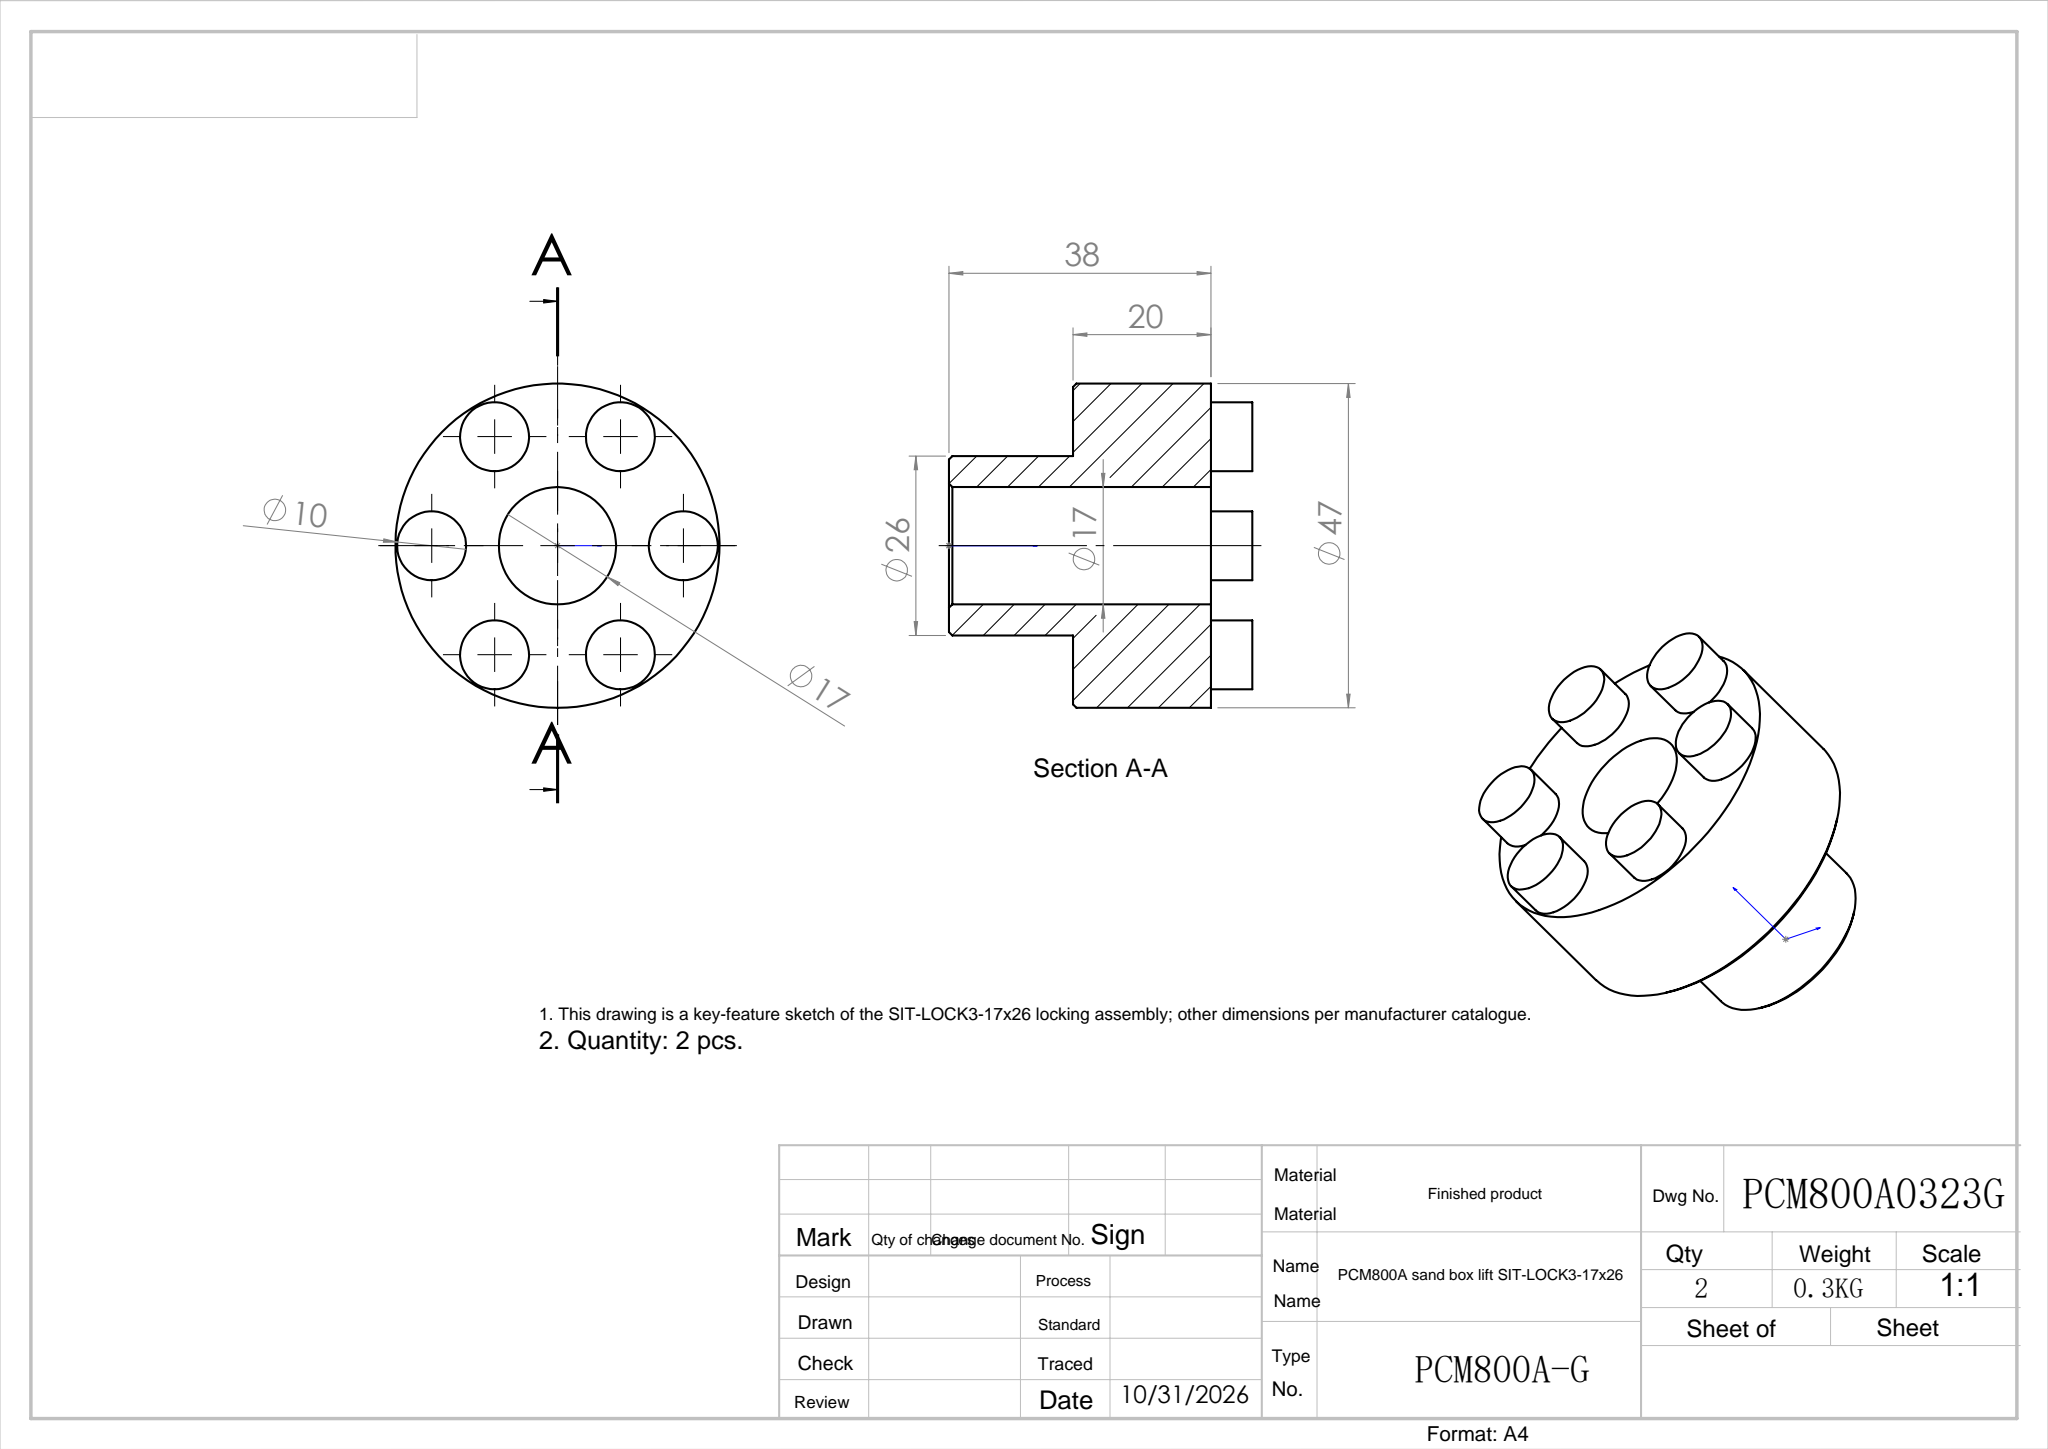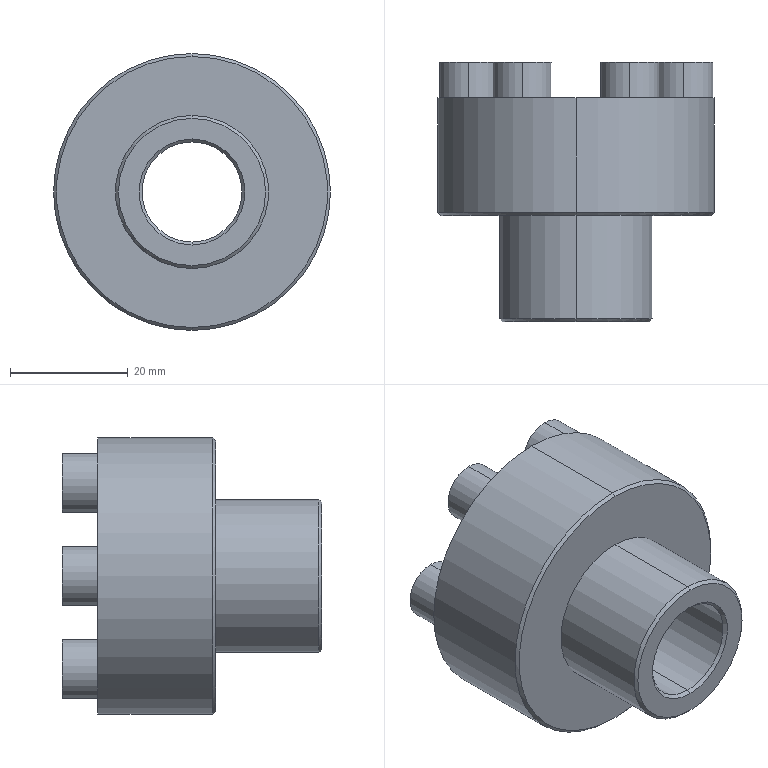Part | SolidWorks | features Boss 2, Chamfer 1, Cut 1, Extrusion 1 | 1 solid | 33 faces | box 47 x 44 x 47 mm | volume 38423 mm3 | cylinder 18 | plane 9 | cone 6 | commonest cylinder face diameters 10 x12 17 x2 26 x2 47 x2
STEP:
#1=CARTESIAN_POINT('',(0.,0.5,8.5));
#2=VERTEX_POINT('',#1);
#3=CARTESIAN_POINT('',(0.,0.5,-8.5));
#4=VERTEX_POINT('',#3);
#5=CARTESIAN_POINT('',(0.,0.5,0.));
#6=DIRECTION('',(0.,-1.,0.));
#7=DIRECTION('',(0.,0.,1.));
#8=AXIS2_PLACEMENT_3D('',#5,#6,#7);
#9=CIRCLE('',#8,8.5);
#10=EDGE_CURVE('',#2,#4,#9,.T.);
#11=ORIENTED_EDGE('',*,*,#10,.F.);
#12=CARTESIAN_POINT('',(0.,0.,9.));
#13=VERTEX_POINT('',#12);
#14=CARTESIAN_POINT('',(0.,0.,9.));
#15=DIRECTION('',(0.,-0.7071,0.7071));
#16=VECTOR('',#15,1000.);
#17=LINE('',#14,#16);
#18=EDGE_CURVE('',#2,#13,#17,.T.);
#19=ORIENTED_EDGE('',*,*,#18,.T.);
#20=CARTESIAN_POINT('',(0.,0.,-9.));
#21=VERTEX_POINT('',#20);
#22=CARTESIAN_POINT('',(0.,0.,0.));
#23=DIRECTION('',(0.,1.,0.));
#24=DIRECTION('',(0.,0.,1.));
#25=AXIS2_PLACEMENT_3D('',#22,#23,#24);
#26=CIRCLE('',#25,9.);
#27=EDGE_CURVE('',#21,#13,#26,.T.);
#28=ORIENTED_EDGE('',*,*,#27,.F.);
#29=CARTESIAN_POINT('',(0.,0.,-9.));
#30=DIRECTION('',(0.,-0.7071,-0.7071));
#31=VECTOR('',#30,1000.);
#32=LINE('',#29,#31);
#33=EDGE_CURVE('',#4,#21,#32,.T.);
#34=ORIENTED_EDGE('',*,*,#33,.F.);
#35=EDGE_LOOP('',(#11,#19,#28,#34));
#36=FACE_OUTER_BOUND('',#35,.T.);
#37=CARTESIAN_POINT('',(0.,0.,0.));
#38=DIRECTION('',(0.,-1.,0.));
#39=DIRECTION('',(0.,0.,-1.));
#40=AXIS2_PLACEMENT_3D('',#37,#38,#39);
#41=CONICAL_SURFACE('',#40,9.,0.7854);
#42=ADVANCED_FACE('',(#36),#41,.F.);
#43=CARTESIAN_POINT('',(0.,0.,-12.5));
#44=VERTEX_POINT('',#43);
#45=CARTESIAN_POINT('',(0.,0.,12.5));
#46=VERTEX_POINT('',#45);
#47=CARTESIAN_POINT('',(0.,0.,0.));
#48=DIRECTION('',(0.,-1.,0.));
#49=DIRECTION('',(0.,0.,1.));
#50=AXIS2_PLACEMENT_3D('',#47,#48,#49);
#51=CIRCLE('',#50,12.5);
#52=EDGE_CURVE('',#44,#46,#51,.T.);
#53=ORIENTED_EDGE('',*,*,#52,.F.);
#54=CARTESIAN_POINT('',(0.,0.5,-13.));
#55=VERTEX_POINT('',#54);
#56=CARTESIAN_POINT('',(0.,0.5,-13.));
#57=DIRECTION('',(0.,0.7071,-0.7071));
#58=VECTOR('',#57,1000.);
#59=LINE('',#56,#58);
#60=EDGE_CURVE('',#44,#55,#59,.T.);
#61=ORIENTED_EDGE('',*,*,#60,.T.);
#62=CARTESIAN_POINT('',(0.,0.5,13.));
#63=VERTEX_POINT('',#62);
#64=CARTESIAN_POINT('',(0.,0.5,0.));
#65=DIRECTION('',(0.,1.,0.));
#66=DIRECTION('',(0.,0.,1.));
#67=AXIS2_PLACEMENT_3D('',#64,#65,#66);
#68=CIRCLE('',#67,13.);
#69=EDGE_CURVE('',#63,#55,#68,.T.);
#70=ORIENTED_EDGE('',*,*,#69,.F.);
#71=CARTESIAN_POINT('',(0.,0.5,13.));
#72=DIRECTION('',(0.,0.7071,0.7071));
#73=VECTOR('',#72,1000.);
#74=LINE('',#71,#73);
#75=EDGE_CURVE('',#46,#63,#74,.T.);
#76=ORIENTED_EDGE('',*,*,#75,.F.);
#77=EDGE_LOOP('',(#53,#61,#70,#76));
#78=FACE_OUTER_BOUND('',#77,.T.);
#79=CARTESIAN_POINT('',(0.,0.5,0.));
#80=DIRECTION('',(0.,1.,0.));
#81=DIRECTION('',(0.,0.,1.));
#82=AXIS2_PLACEMENT_3D('',#79,#80,#81);
#83=CONICAL_SURFACE('',#82,13.,0.7854);
#84=ADVANCED_FACE('',(#78),#83,.T.);
#85=CARTESIAN_POINT('',(0.,18.,-23.));
#86=VERTEX_POINT('',#85);
#87=CARTESIAN_POINT('',(0.,18.,23.));
#88=VERTEX_POINT('',#87);
#89=CARTESIAN_POINT('',(0.,18.,0.));
#90=DIRECTION('',(0.,-1.,0.));
#91=DIRECTION('',(0.,0.,1.));
#92=AXIS2_PLACEMENT_3D('',#89,#90,#91);
#93=CIRCLE('',#92,23.);
#94=EDGE_CURVE('',#86,#88,#93,.T.);
#95=ORIENTED_EDGE('',*,*,#94,.F.);
#96=CARTESIAN_POINT('',(0.,18.5,-23.5));
#97=VERTEX_POINT('',#96);
#98=CARTESIAN_POINT('',(0.,18.5,-23.5));
#99=DIRECTION('',(0.,0.7071,-0.7071));
#100=VECTOR('',#99,1000.);
#101=LINE('',#98,#100);
#102=EDGE_CURVE('',#86,#97,#101,.T.);
#103=ORIENTED_EDGE('',*,*,#102,.T.);
#104=CARTESIAN_POINT('',(0.,18.5,23.5));
#105=VERTEX_POINT('',#104);
#106=CARTESIAN_POINT('',(0.,18.5,0.));
#107=DIRECTION('',(0.,1.,0.));
#108=DIRECTION('',(0.,0.,1.));
#109=AXIS2_PLACEMENT_3D('',#106,#107,#108);
#110=CIRCLE('',#109,23.5);
#111=EDGE_CURVE('',#105,#97,#110,.T.);
#112=ORIENTED_EDGE('',*,*,#111,.F.);
#113=CARTESIAN_POINT('',(0.,18.5,23.5));
#114=DIRECTION('',(0.,0.7071,0.7071));
#115=VECTOR('',#114,1000.);
#116=LINE('',#113,#115);
#117=EDGE_CURVE('',#88,#105,#116,.T.);
#118=ORIENTED_EDGE('',*,*,#117,.F.);
#119=EDGE_LOOP('',(#95,#103,#112,#118));
#120=FACE_OUTER_BOUND('',#119,.T.);
#121=CARTESIAN_POINT('',(0.,18.5,0.));
#122=DIRECTION('',(0.,1.,0.));
#123=DIRECTION('',(0.,0.,1.));
#124=AXIS2_PLACEMENT_3D('',#121,#122,#123);
#125=CONICAL_SURFACE('',#124,23.5,0.7854);
#126=ADVANCED_FACE('',(#120),#125,.T.);
#127=CARTESIAN_POINT('',(9.125,44.,-10.805));
#128=VERTEX_POINT('',#127);
#129=CARTESIAN_POINT('',(9.125,44.,-20.805));
#130=VERTEX_POINT('',#129);
#131=CARTESIAN_POINT('',(9.125,44.,-15.805));
#132=DIRECTION('',(0.,1.,0.));
#133=DIRECTION('',(0.,0.,1.));
#134=AXIS2_PLACEMENT_3D('',#131,#132,#133);
#135=CIRCLE('',#134,5.);
#136=EDGE_CURVE('',#128,#130,#135,.T.);
#137=ORIENTED_EDGE('',*,*,#136,.F.);
#138=CARTESIAN_POINT('',(9.125,38.,-10.805));
#139=VERTEX_POINT('',#138);
#140=CARTESIAN_POINT('',(9.125,44.,-10.805));
#141=DIRECTION('',(0.,-1.,0.));
#142=VECTOR('',#141,1000.);
#143=LINE('',#140,#142);
#144=EDGE_CURVE('',#128,#139,#143,.T.);
#145=ORIENTED_EDGE('',*,*,#144,.T.);
#146=CARTESIAN_POINT('',(9.125,38.,-20.805));
#147=VERTEX_POINT('',#146);
#148=CARTESIAN_POINT('',(9.125,38.,-15.805));
#149=DIRECTION('',(0.,1.,0.));
#150=DIRECTION('',(0.,0.,1.));
#151=AXIS2_PLACEMENT_3D('',#148,#149,#150);
#152=CIRCLE('',#151,5.);
#153=EDGE_CURVE('',#139,#147,#152,.T.);
#154=ORIENTED_EDGE('',*,*,#153,.T.);
#155=CARTESIAN_POINT('',(9.125,44.,-20.805));
#156=DIRECTION('',(0.,-1.,0.));
#157=VECTOR('',#156,1000.);
#158=LINE('',#155,#157);
#159=EDGE_CURVE('',#130,#147,#158,.T.);
#160=ORIENTED_EDGE('',*,*,#159,.F.);
#161=EDGE_LOOP('',(#137,#145,#154,#160));
#162=FACE_OUTER_BOUND('',#161,.T.);
#163=CARTESIAN_POINT('',(9.125,44.,-15.805));
#164=DIRECTION('',(0.,-1.,0.));
#165=DIRECTION('',(0.,0.,-1.));
#166=AXIS2_PLACEMENT_3D('',#163,#164,#165);
#167=CYLINDRICAL_SURFACE('',#166,5.);
#168=ADVANCED_FACE('',(#162),#167,.T.);
#169=CARTESIAN_POINT('',(-9.125,44.,-10.805));
#170=VERTEX_POINT('',#169);
#171=CARTESIAN_POINT('',(-9.125,44.,-20.805));
#172=VERTEX_POINT('',#171);
#173=CARTESIAN_POINT('',(-9.125,44.,-15.805));
#174=DIRECTION('',(0.,1.,0.));
#175=DIRECTION('',(0.,0.,1.));
#176=AXIS2_PLACEMENT_3D('',#173,#174,#175);
#177=CIRCLE('',#176,5.);
#178=EDGE_CURVE('',#170,#172,#177,.T.);
#179=ORIENTED_EDGE('',*,*,#178,.F.);
#180=CARTESIAN_POINT('',(-9.125,38.,-10.805));
#181=VERTEX_POINT('',#180);
#182=CARTESIAN_POINT('',(-9.125,44.,-10.805));
#183=DIRECTION('',(0.,-1.,0.));
#184=VECTOR('',#183,1000.);
#185=LINE('',#182,#184);
#186=EDGE_CURVE('',#170,#181,#185,.T.);
#187=ORIENTED_EDGE('',*,*,#186,.T.);
#188=CARTESIAN_POINT('',(-9.125,38.,-20.805));
#189=VERTEX_POINT('',#188);
#190=CARTESIAN_POINT('',(-9.125,38.,-15.805));
#191=DIRECTION('',(0.,1.,0.));
#192=DIRECTION('',(0.,0.,1.));
#193=AXIS2_PLACEMENT_3D('',#190,#191,#192);
#194=CIRCLE('',#193,5.);
#195=EDGE_CURVE('',#181,#189,#194,.T.);
#196=ORIENTED_EDGE('',*,*,#195,.T.);
#197=CARTESIAN_POINT('',(-9.125,44.,-20.805));
#198=DIRECTION('',(0.,-1.,0.));
#199=VECTOR('',#198,1000.);
#200=LINE('',#197,#199);
#201=EDGE_CURVE('',#172,#189,#200,.T.);
#202=ORIENTED_EDGE('',*,*,#201,.F.);
#203=EDGE_LOOP('',(#179,#187,#196,#202));
#204=FACE_OUTER_BOUND('',#203,.T.);
#205=CARTESIAN_POINT('',(-9.125,44.,-15.805));
#206=DIRECTION('',(0.,-1.,0.));
#207=DIRECTION('',(0.,0.,-1.));
#208=AXIS2_PLACEMENT_3D('',#205,#206,#207);
#209=CYLINDRICAL_SURFACE('',#208,5.);
#210=ADVANCED_FACE('',(#204),#209,.T.);
#211=CARTESIAN_POINT('',(-18.25,44.,5.));
#212=VERTEX_POINT('',#211);
#213=CARTESIAN_POINT('',(-18.25,44.,-5.));
#214=VERTEX_POINT('',#213);
#215=CARTESIAN_POINT('',(-18.25,44.,0.));
#216=DIRECTION('',(0.,1.,0.));
#217=DIRECTION('',(0.,0.,1.));
#218=AXIS2_PLACEMENT_3D('',#215,#216,#217);
#219=CIRCLE('',#218,5.);
#220=EDGE_CURVE('',#212,#214,#219,.T.);
#221=ORIENTED_EDGE('',*,*,#220,.F.);
#222=CARTESIAN_POINT('',(-18.25,38.,5.));
#223=VERTEX_POINT('',#222);
#224=CARTESIAN_POINT('',(-18.25,44.,5.));
#225=DIRECTION('',(0.,-1.,0.));
#226=VECTOR('',#225,1000.);
#227=LINE('',#224,#226);
#228=EDGE_CURVE('',#212,#223,#227,.T.);
#229=ORIENTED_EDGE('',*,*,#228,.T.);
#230=CARTESIAN_POINT('',(-18.25,38.,-5.));
#231=VERTEX_POINT('',#230);
#232=CARTESIAN_POINT('',(-18.25,38.,0.));
#233=DIRECTION('',(0.,1.,0.));
#234=DIRECTION('',(0.,0.,1.));
#235=AXIS2_PLACEMENT_3D('',#232,#233,#234);
#236=CIRCLE('',#235,5.);
#237=EDGE_CURVE('',#223,#231,#236,.T.);
#238=ORIENTED_EDGE('',*,*,#237,.T.);
#239=CARTESIAN_POINT('',(-18.25,44.,-5.));
#240=DIRECTION('',(0.,-1.,0.));
#241=VECTOR('',#240,1000.);
#242=LINE('',#239,#241);
#243=EDGE_CURVE('',#214,#231,#242,.T.);
#244=ORIENTED_EDGE('',*,*,#243,.F.);
#245=EDGE_LOOP('',(#221,#229,#238,#244));
#246=FACE_OUTER_BOUND('',#245,.T.);
#247=CARTESIAN_POINT('',(-18.25,44.,0.));
#248=DIRECTION('',(0.,-1.,0.));
#249=DIRECTION('',(0.,0.,-1.));
#250=AXIS2_PLACEMENT_3D('',#247,#248,#249);
#251=CYLINDRICAL_SURFACE('',#250,5.);
#252=ADVANCED_FACE('',(#246),#251,.T.);
#253=CARTESIAN_POINT('',(-9.125,44.,20.805));
#254=VERTEX_POINT('',#253);
#255=CARTESIAN_POINT('',(-9.125,44.,10.805));
#256=VERTEX_POINT('',#255);
#257=CARTESIAN_POINT('',(-9.125,44.,15.805));
#258=DIRECTION('',(0.,1.,0.));
#259=DIRECTION('',(0.,0.,1.));
#260=AXIS2_PLACEMENT_3D('',#257,#258,#259);
#261=CIRCLE('',#260,5.);
#262=EDGE_CURVE('',#254,#256,#261,.T.);
#263=ORIENTED_EDGE('',*,*,#262,.F.);
#264=CARTESIAN_POINT('',(-9.125,38.,20.805));
#265=VERTEX_POINT('',#264);
#266=CARTESIAN_POINT('',(-9.125,44.,20.805));
#267=DIRECTION('',(0.,-1.,0.));
#268=VECTOR('',#267,1000.);
#269=LINE('',#266,#268);
#270=EDGE_CURVE('',#254,#265,#269,.T.);
#271=ORIENTED_EDGE('',*,*,#270,.T.);
#272=CARTESIAN_POINT('',(-9.125,38.,10.805));
#273=VERTEX_POINT('',#272);
#274=CARTESIAN_POINT('',(-9.125,38.,15.805));
#275=DIRECTION('',(0.,1.,0.));
#276=DIRECTION('',(0.,0.,1.));
#277=AXIS2_PLACEMENT_3D('',#274,#275,#276);
#278=CIRCLE('',#277,5.);
#279=EDGE_CURVE('',#265,#273,#278,.T.);
#280=ORIENTED_EDGE('',*,*,#279,.T.);
#281=CARTESIAN_POINT('',(-9.125,44.,10.805));
#282=DIRECTION('',(0.,-1.,0.));
#283=VECTOR('',#282,1000.);
#284=LINE('',#281,#283);
#285=EDGE_CURVE('',#256,#273,#284,.T.);
#286=ORIENTED_EDGE('',*,*,#285,.F.);
#287=EDGE_LOOP('',(#263,#271,#280,#286));
#288=FACE_OUTER_BOUND('',#287,.T.);
#289=CARTESIAN_POINT('',(-9.125,44.,15.805));
#290=DIRECTION('',(0.,-1.,0.));
#291=DIRECTION('',(0.,0.,-1.));
#292=AXIS2_PLACEMENT_3D('',#289,#290,#291);
#293=CYLINDRICAL_SURFACE('',#292,5.);
#294=ADVANCED_FACE('',(#288),#293,.T.);
#295=CARTESIAN_POINT('',(9.125,44.,20.805));
#296=VERTEX_POINT('',#295);
#297=CARTESIAN_POINT('',(9.125,44.,10.805));
#298=VERTEX_POINT('',#297);
#299=CARTESIAN_POINT('',(9.125,44.,15.805));
#300=DIRECTION('',(0.,1.,0.));
#301=DIRECTION('',(0.,0.,1.));
#302=AXIS2_PLACEMENT_3D('',#299,#300,#301);
#303=CIRCLE('',#302,5.);
#304=EDGE_CURVE('',#296,#298,#303,.T.);
#305=ORIENTED_EDGE('',*,*,#304,.F.);
#306=CARTESIAN_POINT('',(9.125,38.,20.805));
#307=VERTEX_POINT('',#306);
#308=CARTESIAN_POINT('',(9.125,44.,20.805));
#309=DIRECTION('',(0.,-1.,0.));
#310=VECTOR('',#309,1000.);
#311=LINE('',#308,#310);
#312=EDGE_CURVE('',#296,#307,#311,.T.);
#313=ORIENTED_EDGE('',*,*,#312,.T.);
#314=CARTESIAN_POINT('',(9.125,38.,10.805));
#315=VERTEX_POINT('',#314);
#316=CARTESIAN_POINT('',(9.125,38.,15.805));
#317=DIRECTION('',(0.,1.,0.));
#318=DIRECTION('',(0.,0.,1.));
#319=AXIS2_PLACEMENT_3D('',#316,#317,#318);
#320=CIRCLE('',#319,5.);
#321=EDGE_CURVE('',#307,#315,#320,.T.);
#322=ORIENTED_EDGE('',*,*,#321,.T.);
#323=CARTESIAN_POINT('',(9.125,44.,10.805));
#324=DIRECTION('',(0.,-1.,0.));
#325=VECTOR('',#324,1000.);
#326=LINE('',#323,#325);
#327=EDGE_CURVE('',#298,#315,#326,.T.);
#328=ORIENTED_EDGE('',*,*,#327,.F.);
#329=EDGE_LOOP('',(#305,#313,#322,#328));
#330=FACE_OUTER_BOUND('',#329,.T.);
#331=CARTESIAN_POINT('',(9.125,44.,15.805));
#332=DIRECTION('',(0.,-1.,0.));
#333=DIRECTION('',(0.,0.,-1.));
#334=AXIS2_PLACEMENT_3D('',#331,#332,#333);
#335=CYLINDRICAL_SURFACE('',#334,5.);
#336=ADVANCED_FACE('',(#330),#335,.T.);
#337=CARTESIAN_POINT('',(18.25,44.,5.));
#338=VERTEX_POINT('',#337);
#339=CARTESIAN_POINT('',(18.25,44.,-5.));
#340=VERTEX_POINT('',#339);
#341=CARTESIAN_POINT('',(18.25,44.,0.));
#342=DIRECTION('',(0.,1.,0.));
#343=DIRECTION('',(0.,0.,1.));
#344=AXIS2_PLACEMENT_3D('',#341,#342,#343);
#345=CIRCLE('',#344,5.);
#346=EDGE_CURVE('',#338,#340,#345,.T.);
#347=ORIENTED_EDGE('',*,*,#346,.F.);
#348=CARTESIAN_POINT('',(18.25,38.,5.));
#349=VERTEX_POINT('',#348);
#350=CARTESIAN_POINT('',(18.25,44.,5.));
#351=DIRECTION('',(0.,-1.,0.));
#352=VECTOR('',#351,1000.);
#353=LINE('',#350,#352);
#354=EDGE_CURVE('',#338,#349,#353,.T.);
#355=ORIENTED_EDGE('',*,*,#354,.T.);
#356=CARTESIAN_POINT('',(18.25,38.,-5.));
#357=VERTEX_POINT('',#356);
#358=CARTESIAN_POINT('',(18.25,38.,0.));
#359=DIRECTION('',(0.,1.,0.));
#360=DIRECTION('',(0.,0.,1.));
#361=AXIS2_PLACEMENT_3D('',#358,#359,#360);
#362=CIRCLE('',#361,5.);
#363=EDGE_CURVE('',#349,#357,#362,.T.);
#364=ORIENTED_EDGE('',*,*,#363,.T.);
#365=CARTESIAN_POINT('',(18.25,44.,-5.));
#366=DIRECTION('',(0.,-1.,0.));
#367=VECTOR('',#366,1000.);
#368=LINE('',#365,#367);
#369=EDGE_CURVE('',#340,#357,#368,.T.);
#370=ORIENTED_EDGE('',*,*,#369,.F.);
#371=EDGE_LOOP('',(#347,#355,#364,#370));
#372=FACE_OUTER_BOUND('',#371,.T.);
#373=CARTESIAN_POINT('',(18.25,44.,0.));
#374=DIRECTION('',(0.,-1.,0.));
#375=DIRECTION('',(0.,0.,-1.));
#376=AXIS2_PLACEMENT_3D('',#373,#374,#375);
#377=CYLINDRICAL_SURFACE('',#376,5.);
#378=ADVANCED_FACE('',(#372),#377,.T.);
#379=CARTESIAN_POINT('',(0.,38.,23.5));
#380=VERTEX_POINT('',#379);
#381=CARTESIAN_POINT('',(0.,38.,-23.5));
#382=VERTEX_POINT('',#381);
#383=CARTESIAN_POINT('',(0.,38.,0.));
#384=DIRECTION('',(0.,1.,0.));
#385=DIRECTION('',(0.,0.,1.));
#386=AXIS2_PLACEMENT_3D('',#383,#384,#385);
#387=CIRCLE('',#386,23.5);
#388=EDGE_CURVE('',#380,#382,#387,.T.);
#389=ORIENTED_EDGE('',*,*,#388,.F.);
#390=CARTESIAN_POINT('',(0.,38.,23.5));
#391=DIRECTION('',(0.,-1.,0.));
#392=VECTOR('',#391,1000.);
#393=LINE('',#390,#392);
#394=EDGE_CURVE('',#380,#105,#393,.T.);
#395=ORIENTED_EDGE('',*,*,#394,.T.);
#396=ORIENTED_EDGE('',*,*,#111,.T.);
#397=CARTESIAN_POINT('',(0.,38.,-23.5));
#398=DIRECTION('',(0.,-1.,0.));
#399=VECTOR('',#398,1000.);
#400=LINE('',#397,#399);
#401=EDGE_CURVE('',#382,#97,#400,.T.);
#402=ORIENTED_EDGE('',*,*,#401,.F.);
#403=EDGE_LOOP('',(#389,#395,#396,#402));
#404=FACE_OUTER_BOUND('',#403,.T.);
#405=CARTESIAN_POINT('',(0.,38.,0.));
#406=DIRECTION('',(0.,-1.,0.));
#407=DIRECTION('',(0.,0.,-1.));
#408=AXIS2_PLACEMENT_3D('',#405,#406,#407);
#409=CYLINDRICAL_SURFACE('',#408,23.5);
#410=ADVANCED_FACE('',(#404),#409,.T.);
#411=CARTESIAN_POINT('',(0.,38.,8.5));
#412=VERTEX_POINT('',#411);
#413=CARTESIAN_POINT('',(0.,38.,-8.5));
#414=VERTEX_POINT('',#413);
#415=CARTESIAN_POINT('',(0.,38.,0.));
#416=DIRECTION('',(0.,-1.,0.));
#417=DIRECTION('',(0.,0.,-1.));
#418=AXIS2_PLACEMENT_3D('',#415,#416,#417);
#419=CIRCLE('',#418,8.5);
#420=EDGE_CURVE('',#412,#414,#419,.T.);
#421=ORIENTED_EDGE('',*,*,#420,.F.);
#422=CARTESIAN_POINT('',(0.,18.,8.5));
#423=DIRECTION('',(0.,-1.,0.));
#424=VECTOR('',#423,1000.);
#425=LINE('',#422,#424);
#426=EDGE_CURVE('',#412,#2,#425,.T.);
#427=ORIENTED_EDGE('',*,*,#426,.T.);
#428=ORIENTED_EDGE('',*,*,#10,.T.);
#429=CARTESIAN_POINT('',(0.,18.,-8.5));
#430=DIRECTION('',(0.,-1.,0.));
#431=VECTOR('',#430,1000.);
#432=LINE('',#429,#431);
#433=EDGE_CURVE('',#414,#4,#432,.T.);
#434=ORIENTED_EDGE('',*,*,#433,.F.);
#435=EDGE_LOOP('',(#421,#427,#428,#434));
#436=FACE_OUTER_BOUND('',#435,.T.);
#437=CARTESIAN_POINT('',(0.,18.,0.));
#438=DIRECTION('',(0.,-1.,0.));
#439=DIRECTION('',(0.,0.,-1.));
#440=AXIS2_PLACEMENT_3D('',#437,#438,#439);
#441=CYLINDRICAL_SURFACE('',#440,8.5);
#442=ADVANCED_FACE('',(#436),#441,.F.);
#443=CARTESIAN_POINT('',(0.,18.,13.));
#444=VERTEX_POINT('',#443);
#445=CARTESIAN_POINT('',(0.,18.,-13.));
#446=VERTEX_POINT('',#445);
#447=CARTESIAN_POINT('',(0.,18.,0.));
#448=DIRECTION('',(0.,1.,0.));
#449=DIRECTION('',(0.,0.,1.));
#450=AXIS2_PLACEMENT_3D('',#447,#448,#449);
#451=CIRCLE('',#450,13.);
#452=EDGE_CURVE('',#444,#446,#451,.T.);
#453=ORIENTED_EDGE('',*,*,#452,.F.);
#454=CARTESIAN_POINT('',(0.,18.,13.));
#455=DIRECTION('',(0.,-1.,0.));
#456=VECTOR('',#455,1000.);
#457=LINE('',#454,#456);
#458=EDGE_CURVE('',#444,#63,#457,.T.);
#459=ORIENTED_EDGE('',*,*,#458,.T.);
#460=ORIENTED_EDGE('',*,*,#69,.T.);
#461=CARTESIAN_POINT('',(0.,18.,-13.));
#462=DIRECTION('',(0.,-1.,0.));
#463=VECTOR('',#462,1000.);
#464=LINE('',#461,#463);
#465=EDGE_CURVE('',#446,#55,#464,.T.);
#466=ORIENTED_EDGE('',*,*,#465,.F.);
#467=EDGE_LOOP('',(#453,#459,#460,#466));
#468=FACE_OUTER_BOUND('',#467,.T.);
#469=CARTESIAN_POINT('',(0.,18.,0.));
#470=DIRECTION('',(0.,-1.,0.));
#471=DIRECTION('',(0.,0.,-1.));
#472=AXIS2_PLACEMENT_3D('',#469,#470,#471);
#473=CYLINDRICAL_SURFACE('',#472,13.);
#474=ADVANCED_FACE('',(#468),#473,.T.);
#475=CARTESIAN_POINT('',(-9.125,38.,-15.805));
#476=DIRECTION('',(0.,1.,0.));
#477=DIRECTION('',(0.,0.,1.));
#478=AXIS2_PLACEMENT_3D('',#475,#476,#477);
#479=CIRCLE('',#478,5.);
#480=EDGE_CURVE('',#189,#181,#479,.T.);
#481=ORIENTED_EDGE('',*,*,#480,.F.);
#482=ORIENTED_EDGE('',*,*,#195,.F.);
#483=EDGE_LOOP('',(#481,#482));
#484=FACE_BOUND('',#483,.T.);
#485=CARTESIAN_POINT('',(-9.125,38.,15.805));
#486=DIRECTION('',(0.,1.,0.));
#487=DIRECTION('',(0.,0.,1.));
#488=AXIS2_PLACEMENT_3D('',#485,#486,#487);
#489=CIRCLE('',#488,5.);
#490=EDGE_CURVE('',#273,#265,#489,.T.);
#491=ORIENTED_EDGE('',*,*,#490,.F.);
#492=ORIENTED_EDGE('',*,*,#279,.F.);
#493=EDGE_LOOP('',(#491,#492));
#494=FACE_BOUND('',#493,.T.);
#495=CARTESIAN_POINT('',(18.25,38.,0.));
#496=DIRECTION('',(0.,1.,0.));
#497=DIRECTION('',(0.,0.,1.));
#498=AXIS2_PLACEMENT_3D('',#495,#496,#497);
#499=CIRCLE('',#498,5.);
#500=EDGE_CURVE('',#357,#349,#499,.T.);
#501=ORIENTED_EDGE('',*,*,#500,.F.);
#502=ORIENTED_EDGE('',*,*,#363,.F.);
#503=EDGE_LOOP('',(#501,#502));
#504=FACE_BOUND('',#503,.T.);
#505=CARTESIAN_POINT('',(0.,38.,0.));
#506=DIRECTION('',(0.,-1.,0.));
#507=DIRECTION('',(0.,0.,-1.));
#508=AXIS2_PLACEMENT_3D('',#505,#506,#507);
#509=CIRCLE('',#508,8.5);
#510=EDGE_CURVE('',#414,#412,#509,.T.);
#511=ORIENTED_EDGE('',*,*,#510,.T.);
#512=ORIENTED_EDGE('',*,*,#420,.T.);
#513=EDGE_LOOP('',(#511,#512));
#514=FACE_BOUND('',#513,.T.);
#515=CARTESIAN_POINT('',(0.,38.,0.));
#516=DIRECTION('',(0.,1.,0.));
#517=DIRECTION('',(0.,0.,1.));
#518=AXIS2_PLACEMENT_3D('',#515,#516,#517);
#519=CIRCLE('',#518,23.5);
#520=EDGE_CURVE('',#382,#380,#519,.T.);
#521=ORIENTED_EDGE('',*,*,#520,.T.);
#522=ORIENTED_EDGE('',*,*,#388,.T.);
#523=EDGE_LOOP('',(#521,#522));
#524=FACE_OUTER_BOUND('',#523,.T.);
#525=CARTESIAN_POINT('',(9.125,38.,15.805));
#526=DIRECTION('',(0.,1.,0.));
#527=DIRECTION('',(0.,0.,1.));
#528=AXIS2_PLACEMENT_3D('',#525,#526,#527);
#529=CIRCLE('',#528,5.);
#530=EDGE_CURVE('',#315,#307,#529,.T.);
#531=ORIENTED_EDGE('',*,*,#530,.F.);
#532=ORIENTED_EDGE('',*,*,#321,.F.);
#533=EDGE_LOOP('',(#531,#532));
#534=FACE_BOUND('',#533,.T.);
#535=CARTESIAN_POINT('',(-18.25,38.,0.));
#536=DIRECTION('',(0.,1.,0.));
#537=DIRECTION('',(0.,0.,1.));
#538=AXIS2_PLACEMENT_3D('',#535,#536,#537);
#539=CIRCLE('',#538,5.);
#540=EDGE_CURVE('',#231,#223,#539,.T.);
#541=ORIENTED_EDGE('',*,*,#540,.F.);
#542=ORIENTED_EDGE('',*,*,#237,.F.);
#543=EDGE_LOOP('',(#541,#542));
#544=FACE_BOUND('',#543,.T.);
#545=CARTESIAN_POINT('',(9.125,38.,-15.805));
#546=DIRECTION('',(0.,1.,0.));
#547=DIRECTION('',(0.,0.,1.));
#548=AXIS2_PLACEMENT_3D('',#545,#546,#547);
#549=CIRCLE('',#548,5.);
#550=EDGE_CURVE('',#147,#139,#549,.T.);
#551=ORIENTED_EDGE('',*,*,#550,.F.);
#552=ORIENTED_EDGE('',*,*,#153,.F.);
#553=EDGE_LOOP('',(#551,#552));
#554=FACE_BOUND('',#553,.T.);
#555=CARTESIAN_POINT('',(0.,38.,0.));
#556=DIRECTION('',(0.,1.,0.));
#557=DIRECTION('',(0.,0.,1.));
#558=AXIS2_PLACEMENT_3D('',#555,#556,#557);
#559=PLANE('',#558);
#560=ADVANCED_FACE('',(#484,#494,#504,#514,#524,#534,#544,#554),#559,.T.);
#561=CARTESIAN_POINT('',(0.,0.,0.));
#562=DIRECTION('',(0.,-1.,0.));
#563=DIRECTION('',(0.,0.,1.));
#564=AXIS2_PLACEMENT_3D('',#561,#562,#563);
#565=CIRCLE('',#564,12.5);
#566=EDGE_CURVE('',#46,#44,#565,.T.);
#567=ORIENTED_EDGE('',*,*,#566,.T.);
#568=ORIENTED_EDGE('',*,*,#52,.T.);
#569=EDGE_LOOP('',(#567,#568));
#570=FACE_OUTER_BOUND('',#569,.T.);
#571=ORIENTED_EDGE('',*,*,#27,.T.);
#572=CARTESIAN_POINT('',(0.,0.,0.));
#573=DIRECTION('',(0.,1.,0.));
#574=DIRECTION('',(0.,0.,1.));
#575=AXIS2_PLACEMENT_3D('',#572,#573,#574);
#576=CIRCLE('',#575,9.);
#577=EDGE_CURVE('',#13,#21,#576,.T.);
#578=ORIENTED_EDGE('',*,*,#577,.T.);
#579=EDGE_LOOP('',(#571,#578));
#580=FACE_BOUND('',#579,.T.);
#581=CARTESIAN_POINT('',(0.,0.,0.));
#582=DIRECTION('',(0.,1.,0.));
#583=DIRECTION('',(0.,0.,1.));
#584=AXIS2_PLACEMENT_3D('',#581,#582,#583);
#585=PLANE('',#584);
#586=ADVANCED_FACE('',(#570,#580),#585,.F.);
#587=ORIENTED_EDGE('',*,*,#458,.F.);
#588=CARTESIAN_POINT('',(0.,18.,0.));
#589=DIRECTION('',(0.,1.,0.));
#590=DIRECTION('',(0.,0.,1.));
#591=AXIS2_PLACEMENT_3D('',#588,#589,#590);
#592=CIRCLE('',#591,13.);
#593=EDGE_CURVE('',#446,#444,#592,.T.);
#594=ORIENTED_EDGE('',*,*,#593,.F.);
#595=ORIENTED_EDGE('',*,*,#465,.T.);
#596=CARTESIAN_POINT('',(0.,0.5,0.));
#597=DIRECTION('',(0.,1.,0.));
#598=DIRECTION('',(0.,0.,1.));
#599=AXIS2_PLACEMENT_3D('',#596,#597,#598);
#600=CIRCLE('',#599,13.);
#601=EDGE_CURVE('',#55,#63,#600,.T.);
#602=ORIENTED_EDGE('',*,*,#601,.T.);
#603=EDGE_LOOP('',(#587,#594,#595,#602));
#604=FACE_OUTER_BOUND('',#603,.T.);
#605=CARTESIAN_POINT('',(0.,18.,0.));
#606=DIRECTION('',(0.,-1.,0.));
#607=DIRECTION('',(0.,0.,-1.));
#608=AXIS2_PLACEMENT_3D('',#605,#606,#607);
#609=CYLINDRICAL_SURFACE('',#608,13.);
#610=ADVANCED_FACE('',(#604),#609,.T.);
#611=ORIENTED_EDGE('',*,*,#426,.F.);
#612=ORIENTED_EDGE('',*,*,#510,.F.);
#613=ORIENTED_EDGE('',*,*,#433,.T.);
#614=CARTESIAN_POINT('',(0.,0.5,0.));
#615=DIRECTION('',(0.,-1.,0.));
#616=DIRECTION('',(0.,0.,1.));
#617=AXIS2_PLACEMENT_3D('',#614,#615,#616);
#618=CIRCLE('',#617,8.5);
#619=EDGE_CURVE('',#4,#2,#618,.T.);
#620=ORIENTED_EDGE('',*,*,#619,.T.);
#621=EDGE_LOOP('',(#611,#612,#613,#620));
#622=FACE_OUTER_BOUND('',#621,.T.);
#623=CARTESIAN_POINT('',(0.,18.,0.));
#624=DIRECTION('',(0.,-1.,0.));
#625=DIRECTION('',(0.,0.,-1.));
#626=AXIS2_PLACEMENT_3D('',#623,#624,#625);
#627=CYLINDRICAL_SURFACE('',#626,8.5);
#628=ADVANCED_FACE('',(#622),#627,.F.);
#629=CARTESIAN_POINT('',(0.,18.,0.));
#630=DIRECTION('',(0.,-1.,0.));
#631=DIRECTION('',(0.,0.,1.));
#632=AXIS2_PLACEMENT_3D('',#629,#630,#631);
#633=CIRCLE('',#632,23.);
#634=EDGE_CURVE('',#88,#86,#633,.T.);
#635=ORIENTED_EDGE('',*,*,#634,.T.);
#636=ORIENTED_EDGE('',*,*,#94,.T.);
#637=EDGE_LOOP('',(#635,#636));
#638=FACE_OUTER_BOUND('',#637,.T.);
#639=ORIENTED_EDGE('',*,*,#593,.T.);
#640=ORIENTED_EDGE('',*,*,#452,.T.);
#641=EDGE_LOOP('',(#639,#640));
#642=FACE_BOUND('',#641,.T.);
#643=CARTESIAN_POINT('',(0.,18.,0.));
#644=DIRECTION('',(0.,1.,0.));
#645=DIRECTION('',(0.,0.,1.));
#646=AXIS2_PLACEMENT_3D('',#643,#644,#645);
#647=PLANE('',#646);
#648=ADVANCED_FACE('',(#638,#642),#647,.F.);
#649=ORIENTED_EDGE('',*,*,#394,.F.);
#650=ORIENTED_EDGE('',*,*,#520,.F.);
#651=ORIENTED_EDGE('',*,*,#401,.T.);
#652=CARTESIAN_POINT('',(0.,18.5,0.));
#653=DIRECTION('',(0.,1.,0.));
#654=DIRECTION('',(0.,0.,1.));
#655=AXIS2_PLACEMENT_3D('',#652,#653,#654);
#656=CIRCLE('',#655,23.5);
#657=EDGE_CURVE('',#97,#105,#656,.T.);
#658=ORIENTED_EDGE('',*,*,#657,.T.);
#659=EDGE_LOOP('',(#649,#650,#651,#658));
#660=FACE_OUTER_BOUND('',#659,.T.);
#661=CARTESIAN_POINT('',(0.,38.,0.));
#662=DIRECTION('',(0.,-1.,0.));
#663=DIRECTION('',(0.,0.,-1.));
#664=AXIS2_PLACEMENT_3D('',#661,#662,#663);
#665=CYLINDRICAL_SURFACE('',#664,23.5);
#666=ADVANCED_FACE('',(#660),#665,.T.);
#667=ORIENTED_EDGE('',*,*,#354,.F.);
#668=CARTESIAN_POINT('',(18.25,44.,0.));
#669=DIRECTION('',(0.,1.,0.));
#670=DIRECTION('',(0.,0.,1.));
#671=AXIS2_PLACEMENT_3D('',#668,#669,#670);
#672=CIRCLE('',#671,5.);
#673=EDGE_CURVE('',#340,#338,#672,.T.);
#674=ORIENTED_EDGE('',*,*,#673,.F.);
#675=ORIENTED_EDGE('',*,*,#369,.T.);
#676=ORIENTED_EDGE('',*,*,#500,.T.);
#677=EDGE_LOOP('',(#667,#674,#675,#676));
#678=FACE_OUTER_BOUND('',#677,.T.);
#679=CARTESIAN_POINT('',(18.25,44.,0.));
#680=DIRECTION('',(0.,-1.,0.));
#681=DIRECTION('',(0.,0.,-1.));
#682=AXIS2_PLACEMENT_3D('',#679,#680,#681);
#683=CYLINDRICAL_SURFACE('',#682,5.);
#684=ADVANCED_FACE('',(#678),#683,.T.);
#685=ORIENTED_EDGE('',*,*,#673,.T.);
#686=ORIENTED_EDGE('',*,*,#346,.T.);
#687=EDGE_LOOP('',(#685,#686));
#688=FACE_OUTER_BOUND('',#687,.T.);
#689=CARTESIAN_POINT('',(18.25,44.,0.));
#690=DIRECTION('',(0.,1.,0.));
#691=DIRECTION('',(0.,0.,1.));
#692=AXIS2_PLACEMENT_3D('',#689,#690,#691);
#693=PLANE('',#692);
#694=ADVANCED_FACE('',(#688),#693,.T.);
#695=ORIENTED_EDGE('',*,*,#312,.F.);
#696=CARTESIAN_POINT('',(9.125,44.,15.805));
#697=DIRECTION('',(0.,1.,0.));
#698=DIRECTION('',(0.,0.,1.));
#699=AXIS2_PLACEMENT_3D('',#696,#697,#698);
#700=CIRCLE('',#699,5.);
#701=EDGE_CURVE('',#298,#296,#700,.T.);
#702=ORIENTED_EDGE('',*,*,#701,.F.);
#703=ORIENTED_EDGE('',*,*,#327,.T.);
#704=ORIENTED_EDGE('',*,*,#530,.T.);
#705=EDGE_LOOP('',(#695,#702,#703,#704));
#706=FACE_OUTER_BOUND('',#705,.T.);
#707=CARTESIAN_POINT('',(9.125,44.,15.805));
#708=DIRECTION('',(0.,-1.,0.));
#709=DIRECTION('',(0.,0.,-1.));
#710=AXIS2_PLACEMENT_3D('',#707,#708,#709);
#711=CYLINDRICAL_SURFACE('',#710,5.);
#712=ADVANCED_FACE('',(#706),#711,.T.);
#713=ORIENTED_EDGE('',*,*,#701,.T.);
#714=ORIENTED_EDGE('',*,*,#304,.T.);
#715=EDGE_LOOP('',(#713,#714));
#716=FACE_OUTER_BOUND('',#715,.T.);
#717=CARTESIAN_POINT('',(9.125,44.,15.805));
#718=DIRECTION('',(0.,1.,0.));
#719=DIRECTION('',(0.,0.,1.));
#720=AXIS2_PLACEMENT_3D('',#717,#718,#719);
#721=PLANE('',#720);
#722=ADVANCED_FACE('',(#716),#721,.T.);
#723=ORIENTED_EDGE('',*,*,#270,.F.);
#724=CARTESIAN_POINT('',(-9.125,44.,15.805));
#725=DIRECTION('',(0.,1.,0.));
#726=DIRECTION('',(0.,0.,1.));
#727=AXIS2_PLACEMENT_3D('',#724,#725,#726);
#728=CIRCLE('',#727,5.);
#729=EDGE_CURVE('',#256,#254,#728,.T.);
#730=ORIENTED_EDGE('',*,*,#729,.F.);
#731=ORIENTED_EDGE('',*,*,#285,.T.);
#732=ORIENTED_EDGE('',*,*,#490,.T.);
#733=EDGE_LOOP('',(#723,#730,#731,#732));
#734=FACE_OUTER_BOUND('',#733,.T.);
#735=CARTESIAN_POINT('',(-9.125,44.,15.805));
#736=DIRECTION('',(0.,-1.,0.));
#737=DIRECTION('',(0.,0.,-1.));
#738=AXIS2_PLACEMENT_3D('',#735,#736,#737);
#739=CYLINDRICAL_SURFACE('',#738,5.);
#740=ADVANCED_FACE('',(#734),#739,.T.);
#741=ORIENTED_EDGE('',*,*,#729,.T.);
#742=ORIENTED_EDGE('',*,*,#262,.T.);
#743=EDGE_LOOP('',(#741,#742));
#744=FACE_OUTER_BOUND('',#743,.T.);
#745=CARTESIAN_POINT('',(-9.125,44.,15.805));
#746=DIRECTION('',(0.,1.,0.));
#747=DIRECTION('',(0.,0.,1.));
#748=AXIS2_PLACEMENT_3D('',#745,#746,#747);
#749=PLANE('',#748);
#750=ADVANCED_FACE('',(#744),#749,.T.);
#751=ORIENTED_EDGE('',*,*,#228,.F.);
#752=CARTESIAN_POINT('',(-18.25,44.,0.));
#753=DIRECTION('',(0.,1.,0.));
#754=DIRECTION('',(0.,0.,1.));
#755=AXIS2_PLACEMENT_3D('',#752,#753,#754);
#756=CIRCLE('',#755,5.);
#757=EDGE_CURVE('',#214,#212,#756,.T.);
#758=ORIENTED_EDGE('',*,*,#757,.F.);
#759=ORIENTED_EDGE('',*,*,#243,.T.);
#760=ORIENTED_EDGE('',*,*,#540,.T.);
#761=EDGE_LOOP('',(#751,#758,#759,#760));
#762=FACE_OUTER_BOUND('',#761,.T.);
#763=CARTESIAN_POINT('',(-18.25,44.,0.));
#764=DIRECTION('',(0.,-1.,0.));
#765=DIRECTION('',(0.,0.,-1.));
#766=AXIS2_PLACEMENT_3D('',#763,#764,#765);
#767=CYLINDRICAL_SURFACE('',#766,5.);
#768=ADVANCED_FACE('',(#762),#767,.T.);
#769=ORIENTED_EDGE('',*,*,#757,.T.);
#770=ORIENTED_EDGE('',*,*,#220,.T.);
#771=EDGE_LOOP('',(#769,#770));
#772=FACE_OUTER_BOUND('',#771,.T.);
#773=CARTESIAN_POINT('',(-18.25,44.,0.));
#774=DIRECTION('',(0.,1.,0.));
#775=DIRECTION('',(0.,0.,1.));
#776=AXIS2_PLACEMENT_3D('',#773,#774,#775);
#777=PLANE('',#776);
#778=ADVANCED_FACE('',(#772),#777,.T.);
#779=ORIENTED_EDGE('',*,*,#186,.F.);
#780=CARTESIAN_POINT('',(-9.125,44.,-15.805));
#781=DIRECTION('',(0.,1.,0.));
#782=DIRECTION('',(0.,0.,1.));
#783=AXIS2_PLACEMENT_3D('',#780,#781,#782);
#784=CIRCLE('',#783,5.);
#785=EDGE_CURVE('',#172,#170,#784,.T.);
#786=ORIENTED_EDGE('',*,*,#785,.F.);
#787=ORIENTED_EDGE('',*,*,#201,.T.);
#788=ORIENTED_EDGE('',*,*,#480,.T.);
#789=EDGE_LOOP('',(#779,#786,#787,#788));
#790=FACE_OUTER_BOUND('',#789,.T.);
#791=CARTESIAN_POINT('',(-9.125,44.,-15.805));
#792=DIRECTION('',(0.,-1.,0.));
#793=DIRECTION('',(0.,0.,-1.));
#794=AXIS2_PLACEMENT_3D('',#791,#792,#793);
#795=CYLINDRICAL_SURFACE('',#794,5.);
#796=ADVANCED_FACE('',(#790),#795,.T.);
#797=ORIENTED_EDGE('',*,*,#785,.T.);
#798=ORIENTED_EDGE('',*,*,#178,.T.);
#799=EDGE_LOOP('',(#797,#798));
#800=FACE_OUTER_BOUND('',#799,.T.);
#801=CARTESIAN_POINT('',(-9.125,44.,-15.805));
#802=DIRECTION('',(0.,1.,0.));
#803=DIRECTION('',(0.,0.,1.));
#804=AXIS2_PLACEMENT_3D('',#801,#802,#803);
#805=PLANE('',#804);
#806=ADVANCED_FACE('',(#800),#805,.T.);
#807=ORIENTED_EDGE('',*,*,#144,.F.);
#808=CARTESIAN_POINT('',(9.125,44.,-15.805));
#809=DIRECTION('',(0.,1.,0.));
#810=DIRECTION('',(0.,0.,1.));
#811=AXIS2_PLACEMENT_3D('',#808,#809,#810);
#812=CIRCLE('',#811,5.);
#813=EDGE_CURVE('',#130,#128,#812,.T.);
#814=ORIENTED_EDGE('',*,*,#813,.F.);
#815=ORIENTED_EDGE('',*,*,#159,.T.);
#816=ORIENTED_EDGE('',*,*,#550,.T.);
#817=EDGE_LOOP('',(#807,#814,#815,#816));
#818=FACE_OUTER_BOUND('',#817,.T.);
#819=CARTESIAN_POINT('',(9.125,44.,-15.805));
#820=DIRECTION('',(0.,-1.,0.));
#821=DIRECTION('',(0.,0.,-1.));
#822=AXIS2_PLACEMENT_3D('',#819,#820,#821);
#823=CYLINDRICAL_SURFACE('',#822,5.);
#824=ADVANCED_FACE('',(#818),#823,.T.);
#825=ORIENTED_EDGE('',*,*,#813,.T.);
#826=ORIENTED_EDGE('',*,*,#136,.T.);
#827=EDGE_LOOP('',(#825,#826));
#828=FACE_OUTER_BOUND('',#827,.T.);
#829=CARTESIAN_POINT('',(9.125,44.,-15.805));
#830=DIRECTION('',(0.,1.,0.));
#831=DIRECTION('',(0.,0.,1.));
#832=AXIS2_PLACEMENT_3D('',#829,#830,#831);
#833=PLANE('',#832);
#834=ADVANCED_FACE('',(#828),#833,.T.);
#835=ORIENTED_EDGE('',*,*,#102,.F.);
#836=ORIENTED_EDGE('',*,*,#634,.F.);
#837=ORIENTED_EDGE('',*,*,#117,.T.);
#838=ORIENTED_EDGE('',*,*,#657,.F.);
#839=EDGE_LOOP('',(#835,#836,#837,#838));
#840=FACE_OUTER_BOUND('',#839,.T.);
#841=CARTESIAN_POINT('',(0.,18.5,0.));
#842=DIRECTION('',(0.,1.,0.));
#843=DIRECTION('',(0.,0.,1.));
#844=AXIS2_PLACEMENT_3D('',#841,#842,#843);
#845=CONICAL_SURFACE('',#844,23.5,0.7854);
#846=ADVANCED_FACE('',(#840),#845,.T.);
#847=ORIENTED_EDGE('',*,*,#60,.F.);
#848=ORIENTED_EDGE('',*,*,#566,.F.);
#849=ORIENTED_EDGE('',*,*,#75,.T.);
#850=ORIENTED_EDGE('',*,*,#601,.F.);
#851=EDGE_LOOP('',(#847,#848,#849,#850));
#852=FACE_OUTER_BOUND('',#851,.T.);
#853=CARTESIAN_POINT('',(0.,0.5,0.));
#854=DIRECTION('',(0.,1.,0.));
#855=DIRECTION('',(0.,0.,1.));
#856=AXIS2_PLACEMENT_3D('',#853,#854,#855);
#857=CONICAL_SURFACE('',#856,13.,0.7854);
#858=ADVANCED_FACE('',(#852),#857,.T.);
#859=ORIENTED_EDGE('',*,*,#18,.F.);
#860=ORIENTED_EDGE('',*,*,#619,.F.);
#861=ORIENTED_EDGE('',*,*,#33,.T.);
#862=ORIENTED_EDGE('',*,*,#577,.F.);
#863=EDGE_LOOP('',(#859,#860,#861,#862));
#864=FACE_OUTER_BOUND('',#863,.T.);
#865=CARTESIAN_POINT('',(0.,0.,0.));
#866=DIRECTION('',(0.,-1.,0.));
#867=DIRECTION('',(0.,0.,-1.));
#868=AXIS2_PLACEMENT_3D('',#865,#866,#867);
#869=CONICAL_SURFACE('',#868,9.,0.7854);
#870=ADVANCED_FACE('',(#864),#869,.F.);
#871=CLOSED_SHELL('',(#42,#84,#126,#168,#210,#252,#294,#336,#378,#410,#442,#474,#560,#586,#610,#628,#648,#666,#684,#694,#712,#722,#740,#750,#768,#778,#796,#806,#824,#834,#846,#858,#870));
#872=MANIFOLD_SOLID_BREP('',#871);
#873=CARTESIAN_POINT('',(0.,0.,0.));
#874=DIRECTION('',(0.,0.,1.));
#875=DIRECTION('',(1.,0.,0.));
#876=AXIS2_PLACEMENT_3D('',#873,#874,#875);
#877=(LENGTH_UNIT()NAMED_UNIT(*)SI_UNIT(.MILLI.,.METRE.));
#878=UNCERTAINTY_MEASURE_WITH_UNIT(LENGTH_MEASURE(0.00001),#877,'','');
#879=(NAMED_UNIT(*)PLANE_ANGLE_UNIT()SI_UNIT($,.RADIAN.));
#880=(NAMED_UNIT(*)SI_UNIT($,.STERADIAN.)SOLID_ANGLE_UNIT());
#881=(GEOMETRIC_REPRESENTATION_CONTEXT(3)GLOBAL_UNCERTAINTY_ASSIGNED_CONTEXT((#878))GLOBAL_UNIT_ASSIGNED_CONTEXT((#877,#879,#880))REPRESENTATION_CONTEXT('',''));
#882=ADVANCED_BREP_SHAPE_REPRESENTATION('',(#872,#876),#881);